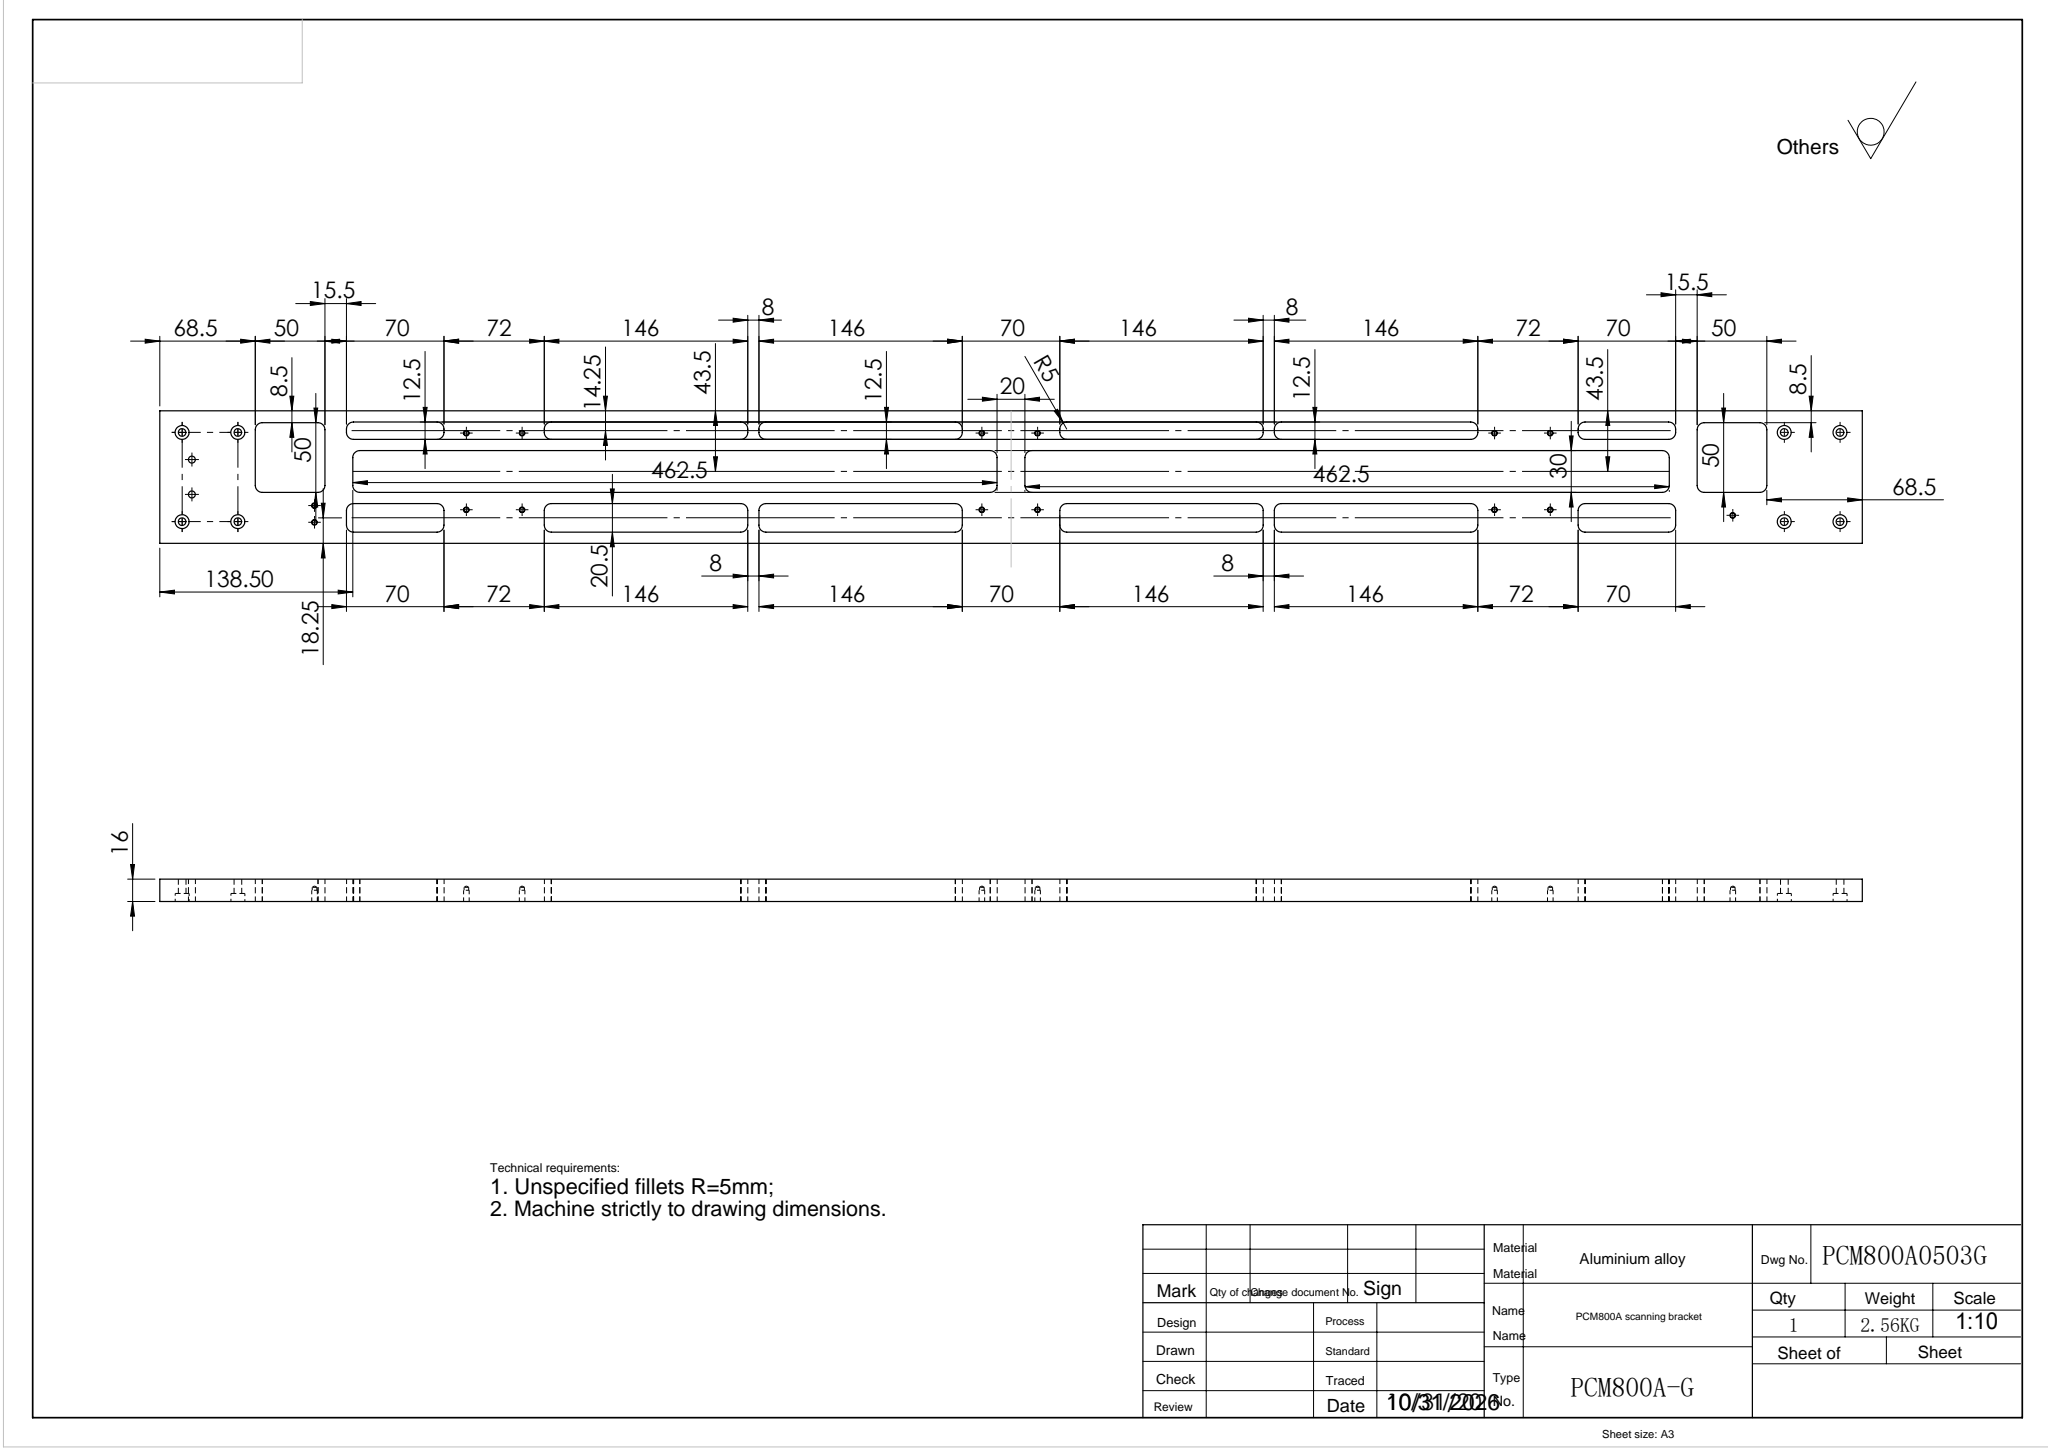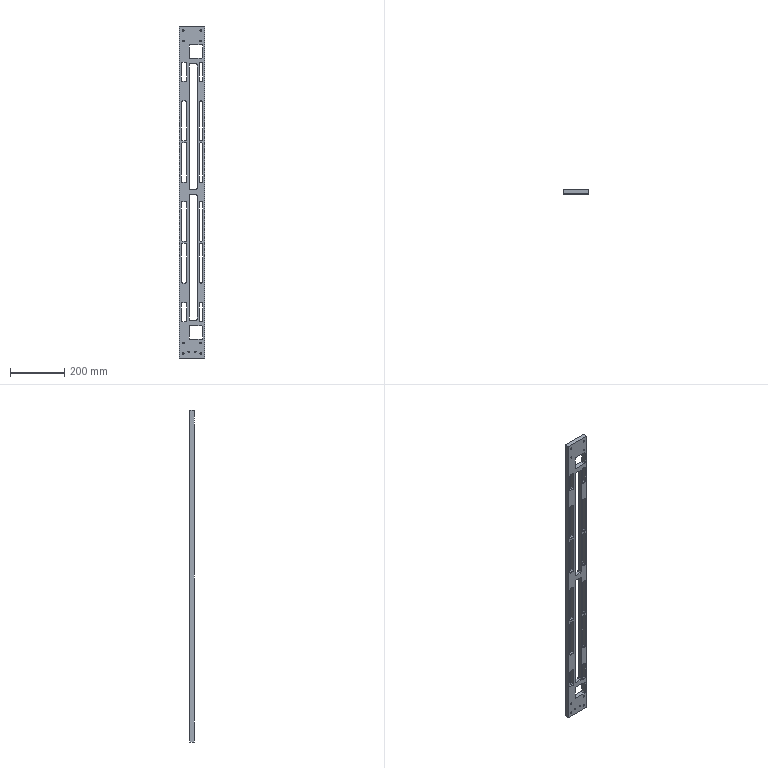Part | SolidWorks | features HoleWzd 3, 3DProfileFeature 2, LPattern 2, Extrusion 1, Fillet 1, ICE 1 | 1 solid | 283 faces | box 95 x 16 x 1222 mm | volume 948675 mm3 | cylinder 160 | plane 93 | cone 30 | commonest cylinder face diameters 10 x80 3.3 x30 4 x30 5.5 x16 5 x4